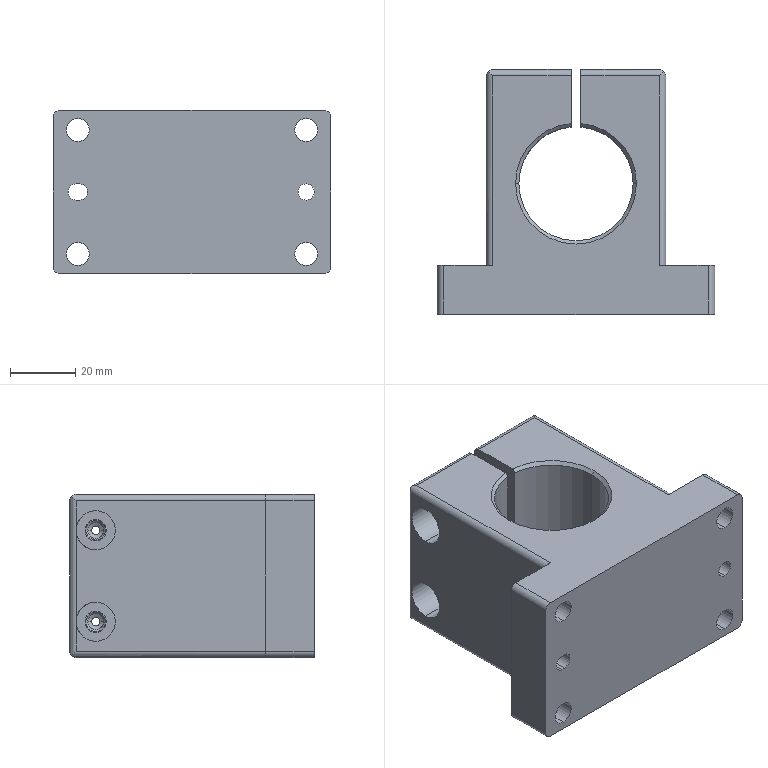Part | SolidWorks | features BaseBody 1 | 1 solid | 72 faces | box 85 x 75 x 50 mm | volume 169404 mm3 | cylinder 41 | plane 17 | cone 14 | commonest cylinder face diameters 4 x14 7 x8 4.917 x4 5 x4 6.5 x4 12 x4